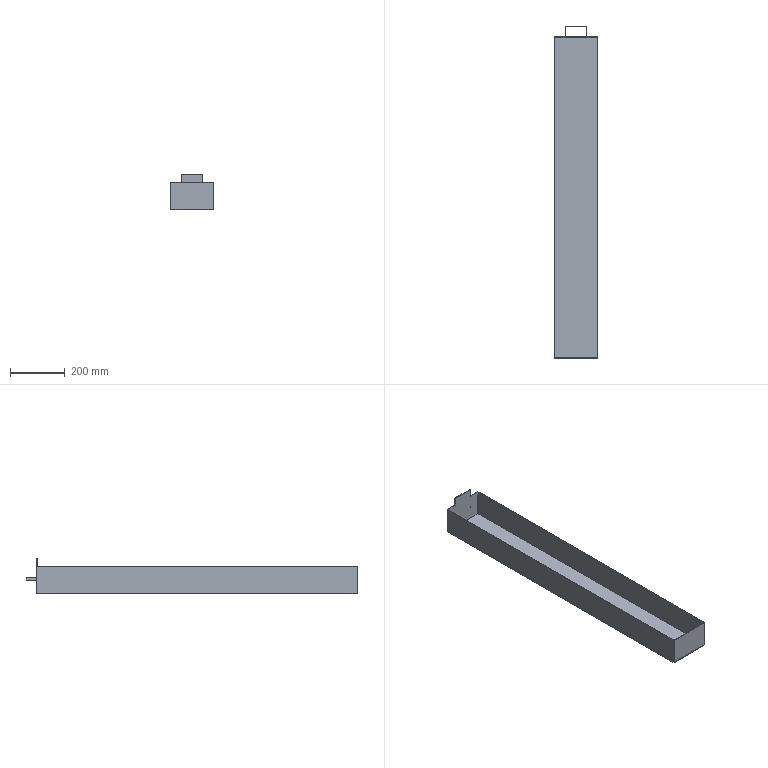Part | NX | features solid 2 | 1 solid | 22 faces | box 160 x 1212 x 130 mm | volume 903536 mm3 | plane 22
STEP:
#1=CARTESIAN_POINT('',(-370.,1107.,-565.));
#2=VERTEX_POINT('',#1);
#3=CARTESIAN_POINT('',(-370.,1107.,-465.));
#4=VERTEX_POINT('',#3);
#5=CARTESIAN_POINT('',(-370.,1107.,-565.));
#6=DIRECTION('',(0.,0.,1.));
#7=VECTOR('',#6,1000.);
#8=LINE('',#5,#7);
#9=EDGE_CURVE('',#2,#4,#8,.T.);
#10=ORIENTED_EDGE('',*,*,#9,.T.);
#11=CARTESIAN_POINT('',(-370.,-65.,-465.));
#12=VERTEX_POINT('',#11);
#13=CARTESIAN_POINT('',(-370.,807.,-465.));
#14=DIRECTION('',(0.,1.,0.));
#15=VECTOR('',#14,1000.);
#16=LINE('',#13,#15);
#17=EDGE_CURVE('',#12,#4,#16,.T.);
#18=ORIENTED_EDGE('',*,*,#17,.F.);
#19=CARTESIAN_POINT('',(-370.,-65.,-565.));
#20=VERTEX_POINT('',#19);
#21=CARTESIAN_POINT('',(-370.,-65.,-565.));
#22=DIRECTION('',(0.,0.,-1.));
#23=VECTOR('',#22,1000.);
#24=LINE('',#21,#23);
#25=EDGE_CURVE('',#20,#12,#24,.F.);
#26=ORIENTED_EDGE('',*,*,#25,.F.);
#27=CARTESIAN_POINT('',(-370.,807.,-565.));
#28=DIRECTION('',(0.,1.,0.));
#29=VECTOR('',#28,1000.);
#30=LINE('',#27,#29);
#31=EDGE_CURVE('',#20,#2,#30,.T.);
#32=ORIENTED_EDGE('',*,*,#31,.T.);
#33=EDGE_LOOP('',(#10,#18,#26,#32));
#34=FACE_BOUND('',#33,.T.);
#35=CARTESIAN_POINT('',(-370.,807.,-565.));
#36=DIRECTION('',(-1.,0.,0.));
#37=DIRECTION('',(0.,1.,0.));
#38=AXIS2_PLACEMENT_3D('',#35,#36,#37);
#39=PLANE('',#38);
#40=ADVANCED_FACE('',(#34),#39,.F.);
#41=CARTESIAN_POINT('',(-490.,1107.,-505.));
#42=VERTEX_POINT('',#41);
#43=CARTESIAN_POINT('',(-490.,1107.,-515.));
#44=VERTEX_POINT('',#43);
#45=CARTESIAN_POINT('',(-490.,1107.,-565.));
#46=DIRECTION('',(0.,0.,-1.));
#47=VECTOR('',#46,1000.);
#48=LINE('',#45,#47);
#49=EDGE_CURVE('',#42,#44,#48,.T.);
#50=ORIENTED_EDGE('',*,*,#49,.T.);
#51=CARTESIAN_POINT('',(-488.,1107.,-515.));
#52=VERTEX_POINT('',#51);
#53=CARTESIAN_POINT('',(-410.,1107.,-515.));
#54=DIRECTION('',(1.,0.,0.));
#55=VECTOR('',#54,1000.);
#56=LINE('',#53,#55);
#57=EDGE_CURVE('',#52,#44,#56,.F.);
#58=ORIENTED_EDGE('',*,*,#57,.F.);
#59=CARTESIAN_POINT('',(-488.,1107.,-505.));
#60=VERTEX_POINT('',#59);
#61=CARTESIAN_POINT('',(-488.,1107.,-565.));
#62=DIRECTION('',(0.,0.,-1.));
#63=VECTOR('',#62,1000.);
#64=LINE('',#61,#63);
#65=EDGE_CURVE('',#60,#52,#64,.T.);
#66=ORIENTED_EDGE('',*,*,#65,.F.);
#67=CARTESIAN_POINT('',(-410.,1107.,-505.));
#68=DIRECTION('',(1.,0.,0.));
#69=VECTOR('',#68,1000.);
#70=LINE('',#67,#69);
#71=EDGE_CURVE('',#60,#42,#70,.F.);
#72=ORIENTED_EDGE('',*,*,#71,.T.);
#73=EDGE_LOOP('',(#50,#58,#66,#72));
#74=FACE_BOUND('',#73,.T.);
#75=CARTESIAN_POINT('',(-412.,1107.,-505.));
#76=VERTEX_POINT('',#75);
#77=CARTESIAN_POINT('',(-412.,1107.,-515.));
#78=VERTEX_POINT('',#77);
#79=CARTESIAN_POINT('',(-412.,1107.,-565.));
#80=DIRECTION('',(0.,0.,1.));
#81=VECTOR('',#80,1000.);
#82=LINE('',#79,#81);
#83=EDGE_CURVE('',#76,#78,#82,.F.);
#84=ORIENTED_EDGE('',*,*,#83,.T.);
#85=CARTESIAN_POINT('',(-410.,1107.,-515.));
#86=VERTEX_POINT('',#85);
#87=CARTESIAN_POINT('',(-410.,1107.,-515.));
#88=DIRECTION('',(1.,0.,0.));
#89=VECTOR('',#88,1000.);
#90=LINE('',#87,#89);
#91=EDGE_CURVE('',#86,#78,#90,.F.);
#92=ORIENTED_EDGE('',*,*,#91,.F.);
#93=CARTESIAN_POINT('',(-410.,1107.,-505.));
#94=VERTEX_POINT('',#93);
#95=CARTESIAN_POINT('',(-410.,1107.,-565.));
#96=DIRECTION('',(0.,0.,-1.));
#97=VECTOR('',#96,1000.);
#98=LINE('',#95,#97);
#99=EDGE_CURVE('',#94,#86,#98,.T.);
#100=ORIENTED_EDGE('',*,*,#99,.F.);
#101=CARTESIAN_POINT('',(-410.,1107.,-505.));
#102=DIRECTION('',(1.,0.,0.));
#103=VECTOR('',#102,1000.);
#104=LINE('',#101,#103);
#105=EDGE_CURVE('',#94,#76,#104,.F.);
#106=ORIENTED_EDGE('',*,*,#105,.T.);
#107=EDGE_LOOP('',(#84,#92,#100,#106));
#108=FACE_BOUND('',#107,.T.);
#109=CARTESIAN_POINT('',(-410.,1107.,-465.));
#110=VERTEX_POINT('',#109);
#111=CARTESIAN_POINT('',(-375.,1107.,-465.));
#112=DIRECTION('',(-1.,0.,0.));
#113=VECTOR('',#112,1000.);
#114=LINE('',#111,#113);
#115=EDGE_CURVE('',#4,#110,#114,.T.);
#116=ORIENTED_EDGE('',*,*,#115,.F.);
#117=ORIENTED_EDGE('',*,*,#9,.F.);
#118=CARTESIAN_POINT('',(-530.,1107.,-565.));
#119=VERTEX_POINT('',#118);
#120=CARTESIAN_POINT('',(-375.,1107.,-565.));
#121=DIRECTION('',(-1.,0.,0.));
#122=VECTOR('',#121,1000.);
#123=LINE('',#120,#122);
#124=EDGE_CURVE('',#2,#119,#123,.T.);
#125=ORIENTED_EDGE('',*,*,#124,.T.);
#126=CARTESIAN_POINT('',(-530.,1107.,-465.));
#127=VERTEX_POINT('',#126);
#128=CARTESIAN_POINT('',(-530.,1107.,-565.));
#129=DIRECTION('',(0.,0.,-1.));
#130=VECTOR('',#129,1000.);
#131=LINE('',#128,#130);
#132=EDGE_CURVE('',#119,#127,#131,.F.);
#133=ORIENTED_EDGE('',*,*,#132,.T.);
#134=CARTESIAN_POINT('',(-490.,1107.,-465.));
#135=VERTEX_POINT('',#134);
#136=CARTESIAN_POINT('',(-375.,1107.,-465.));
#137=DIRECTION('',(-1.,0.,0.));
#138=VECTOR('',#137,1000.);
#139=LINE('',#136,#138);
#140=EDGE_CURVE('',#135,#127,#139,.T.);
#141=ORIENTED_EDGE('',*,*,#140,.F.);
#142=CARTESIAN_POINT('',(-490.,1107.,-435.));
#143=VERTEX_POINT('',#142);
#144=CARTESIAN_POINT('',(-490.,1107.,-565.));
#145=DIRECTION('',(0.,0.,-1.));
#146=VECTOR('',#145,1000.);
#147=LINE('',#144,#146);
#148=EDGE_CURVE('',#135,#143,#147,.F.);
#149=ORIENTED_EDGE('',*,*,#148,.T.);
#150=CARTESIAN_POINT('',(-410.,1107.,-435.));
#151=VERTEX_POINT('',#150);
#152=CARTESIAN_POINT('',(-370.,1107.,-435.));
#153=DIRECTION('',(-1.,0.,0.));
#154=VECTOR('',#153,1000.);
#155=LINE('',#152,#154);
#156=EDGE_CURVE('',#151,#143,#155,.T.);
#157=ORIENTED_EDGE('',*,*,#156,.F.);
#158=CARTESIAN_POINT('',(-410.,1107.,-565.));
#159=DIRECTION('',(0.,0.,1.));
#160=VECTOR('',#159,1000.);
#161=LINE('',#158,#160);
#162=EDGE_CURVE('',#110,#151,#161,.T.);
#163=ORIENTED_EDGE('',*,*,#162,.F.);
#164=EDGE_LOOP('',(#116,#117,#125,#133,#141,#149,#157,#163));
#165=FACE_BOUND('',#164,.T.);
#166=CARTESIAN_POINT('',(-375.,1107.,-565.));
#167=DIRECTION('',(0.,-1.,0.));
#168=DIRECTION('',(-1.,0.,0.));
#169=AXIS2_PLACEMENT_3D('',#166,#167,#168);
#170=PLANE('',#169);
#171=ADVANCED_FACE('',(#74,#108,#165),#170,.F.);
#172=CARTESIAN_POINT('',(-530.,-65.,-465.));
#173=VERTEX_POINT('',#172);
#174=CARTESIAN_POINT('',(-530.,807.,-465.));
#175=DIRECTION('',(0.,-1.,0.));
#176=VECTOR('',#175,1000.);
#177=LINE('',#174,#176);
#178=EDGE_CURVE('',#173,#127,#177,.F.);
#179=ORIENTED_EDGE('',*,*,#178,.T.);
#180=ORIENTED_EDGE('',*,*,#132,.F.);
#181=CARTESIAN_POINT('',(-530.,-65.,-565.));
#182=VERTEX_POINT('',#181);
#183=CARTESIAN_POINT('',(-530.,807.,-565.));
#184=DIRECTION('',(0.,-1.,0.));
#185=VECTOR('',#184,1000.);
#186=LINE('',#183,#185);
#187=EDGE_CURVE('',#182,#119,#186,.F.);
#188=ORIENTED_EDGE('',*,*,#187,.F.);
#189=CARTESIAN_POINT('',(-530.,-65.,-565.));
#190=DIRECTION('',(0.,0.,1.));
#191=VECTOR('',#190,1000.);
#192=LINE('',#189,#191);
#193=EDGE_CURVE('',#182,#173,#192,.T.);
#194=ORIENTED_EDGE('',*,*,#193,.T.);
#195=EDGE_LOOP('',(#179,#180,#188,#194));
#196=FACE_BOUND('',#195,.T.);
#197=CARTESIAN_POINT('',(-530.,807.,-565.));
#198=DIRECTION('',(-1.,0.,0.));
#199=DIRECTION('',(0.,1.,0.));
#200=AXIS2_PLACEMENT_3D('',#197,#198,#199);
#201=PLANE('',#200);
#202=ADVANCED_FACE('',(#196),#201,.T.);
#203=CARTESIAN_POINT('',(-372.,1105.,-563.));
#204=VERTEX_POINT('',#203);
#205=CARTESIAN_POINT('',(-372.,1105.,-465.));
#206=VERTEX_POINT('',#205);
#207=CARTESIAN_POINT('',(-372.,1105.,-565.));
#208=DIRECTION('',(0.,0.,1.));
#209=VECTOR('',#208,1000.);
#210=LINE('',#207,#209);
#211=EDGE_CURVE('',#204,#206,#210,.T.);
#212=ORIENTED_EDGE('',*,*,#211,.T.);
#213=CARTESIAN_POINT('',(-410.,1105.,-465.));
#214=VERTEX_POINT('',#213);
#215=CARTESIAN_POINT('',(-375.,1105.,-465.));
#216=DIRECTION('',(-1.,0.,0.));
#217=VECTOR('',#216,1000.);
#218=LINE('',#215,#217);
#219=EDGE_CURVE('',#206,#214,#218,.T.);
#220=ORIENTED_EDGE('',*,*,#219,.T.);
#221=CARTESIAN_POINT('',(-410.,1105.,-435.));
#222=VERTEX_POINT('',#221);
#223=CARTESIAN_POINT('',(-410.,1105.,-565.));
#224=DIRECTION('',(0.,0.,1.));
#225=VECTOR('',#224,1000.);
#226=LINE('',#223,#225);
#227=EDGE_CURVE('',#214,#222,#226,.T.);
#228=ORIENTED_EDGE('',*,*,#227,.T.);
#229=CARTESIAN_POINT('',(-490.,1105.,-435.));
#230=VERTEX_POINT('',#229);
#231=CARTESIAN_POINT('',(-370.,1105.,-435.));
#232=DIRECTION('',(-1.,0.,0.));
#233=VECTOR('',#232,1000.);
#234=LINE('',#231,#233);
#235=EDGE_CURVE('',#222,#230,#234,.T.);
#236=ORIENTED_EDGE('',*,*,#235,.T.);
#237=CARTESIAN_POINT('',(-490.,1105.,-465.));
#238=VERTEX_POINT('',#237);
#239=CARTESIAN_POINT('',(-490.,1105.,-565.));
#240=DIRECTION('',(0.,0.,-1.));
#241=VECTOR('',#240,1000.);
#242=LINE('',#239,#241);
#243=EDGE_CURVE('',#238,#230,#242,.F.);
#244=ORIENTED_EDGE('',*,*,#243,.F.);
#245=CARTESIAN_POINT('',(-528.,1105.,-465.));
#246=VERTEX_POINT('',#245);
#247=CARTESIAN_POINT('',(-375.,1105.,-465.));
#248=DIRECTION('',(-1.,0.,0.));
#249=VECTOR('',#248,1000.);
#250=LINE('',#247,#249);
#251=EDGE_CURVE('',#238,#246,#250,.T.);
#252=ORIENTED_EDGE('',*,*,#251,.T.);
#253=CARTESIAN_POINT('',(-528.,1105.,-563.));
#254=VERTEX_POINT('',#253);
#255=CARTESIAN_POINT('',(-528.,1105.,-565.));
#256=DIRECTION('',(0.,0.,-1.));
#257=VECTOR('',#256,1000.);
#258=LINE('',#255,#257);
#259=EDGE_CURVE('',#254,#246,#258,.F.);
#260=ORIENTED_EDGE('',*,*,#259,.F.);
#261=CARTESIAN_POINT('',(-375.,1105.,-563.));
#262=DIRECTION('',(-1.,0.,0.));
#263=VECTOR('',#262,1000.);
#264=LINE('',#261,#263);
#265=EDGE_CURVE('',#204,#254,#264,.T.);
#266=ORIENTED_EDGE('',*,*,#265,.F.);
#267=EDGE_LOOP('',(#212,#220,#228,#236,#244,#252,#260,#266));
#268=FACE_BOUND('',#267,.T.);
#269=CARTESIAN_POINT('',(-375.,1105.,-565.));
#270=DIRECTION('',(0.,-1.,0.));
#271=DIRECTION('',(-1.,0.,0.));
#272=AXIS2_PLACEMENT_3D('',#269,#270,#271);
#273=PLANE('',#272);
#274=ADVANCED_FACE('',(#268),#273,.T.);
#275=CARTESIAN_POINT('',(-490.,807.,-465.));
#276=DIRECTION('',(0.,1.,0.));
#277=VECTOR('',#276,1000.);
#278=LINE('',#275,#277);
#279=EDGE_CURVE('',#135,#238,#278,.F.);
#280=ORIENTED_EDGE('',*,*,#279,.F.);
#281=ORIENTED_EDGE('',*,*,#140,.T.);
#282=ORIENTED_EDGE('',*,*,#178,.F.);
#283=CARTESIAN_POINT('',(-375.,-65.,-465.));
#284=DIRECTION('',(1.,0.,0.));
#285=VECTOR('',#284,1000.);
#286=LINE('',#283,#285);
#287=EDGE_CURVE('',#12,#173,#286,.F.);
#288=ORIENTED_EDGE('',*,*,#287,.F.);
#289=ORIENTED_EDGE('',*,*,#17,.T.);
#290=ORIENTED_EDGE('',*,*,#115,.T.);
#291=CARTESIAN_POINT('',(-410.,807.,-465.));
#292=DIRECTION('',(0.,1.,0.));
#293=VECTOR('',#292,1000.);
#294=LINE('',#291,#293);
#295=EDGE_CURVE('',#214,#110,#294,.T.);
#296=ORIENTED_EDGE('',*,*,#295,.F.);
#297=ORIENTED_EDGE('',*,*,#219,.F.);
#298=CARTESIAN_POINT('',(-372.,-63.,-465.));
#299=VERTEX_POINT('',#298);
#300=CARTESIAN_POINT('',(-372.,807.,-465.));
#301=DIRECTION('',(0.,1.,0.));
#302=VECTOR('',#301,1000.);
#303=LINE('',#300,#302);
#304=EDGE_CURVE('',#299,#206,#303,.T.);
#305=ORIENTED_EDGE('',*,*,#304,.F.);
#306=CARTESIAN_POINT('',(-528.,-63.,-465.));
#307=VERTEX_POINT('',#306);
#308=CARTESIAN_POINT('',(-375.,-63.,-465.));
#309=DIRECTION('',(1.,0.,0.));
#310=VECTOR('',#309,1000.);
#311=LINE('',#308,#310);
#312=EDGE_CURVE('',#299,#307,#311,.F.);
#313=ORIENTED_EDGE('',*,*,#312,.T.);
#314=CARTESIAN_POINT('',(-528.,807.,-465.));
#315=DIRECTION('',(0.,-1.,0.));
#316=VECTOR('',#315,1000.);
#317=LINE('',#314,#316);
#318=EDGE_CURVE('',#307,#246,#317,.F.);
#319=ORIENTED_EDGE('',*,*,#318,.T.);
#320=ORIENTED_EDGE('',*,*,#251,.F.);
#321=EDGE_LOOP('',(#280,#281,#282,#288,#289,#290,#296,#297,#305,#313,#319,#320));
#322=FACE_BOUND('',#321,.T.);
#323=CARTESIAN_POINT('',(-375.,807.,-465.));
#324=DIRECTION('',(0.,0.,1.));
#325=DIRECTION('',(1.,0.,0.));
#326=AXIS2_PLACEMENT_3D('',#323,#324,#325);
#327=PLANE('',#326);
#328=ADVANCED_FACE('',(#322),#327,.T.);
#329=ORIENTED_EDGE('',*,*,#31,.F.);
#330=CARTESIAN_POINT('',(-375.,-65.,-565.));
#331=DIRECTION('',(1.,0.,0.));
#332=VECTOR('',#331,1000.);
#333=LINE('',#330,#332);
#334=EDGE_CURVE('',#20,#182,#333,.F.);
#335=ORIENTED_EDGE('',*,*,#334,.T.);
#336=ORIENTED_EDGE('',*,*,#187,.T.);
#337=ORIENTED_EDGE('',*,*,#124,.F.);
#338=EDGE_LOOP('',(#329,#335,#336,#337));
#339=FACE_BOUND('',#338,.T.);
#340=CARTESIAN_POINT('',(-375.,807.,-565.));
#341=DIRECTION('',(0.,0.,1.));
#342=DIRECTION('',(1.,0.,0.));
#343=AXIS2_PLACEMENT_3D('',#340,#341,#342);
#344=PLANE('',#343);
#345=ADVANCED_FACE('',(#339),#344,.F.);
#346=CARTESIAN_POINT('',(-372.,-63.,-563.));
#347=VERTEX_POINT('',#346);
#348=CARTESIAN_POINT('',(-372.,807.,-563.));
#349=DIRECTION('',(0.,1.,0.));
#350=VECTOR('',#349,1000.);
#351=LINE('',#348,#350);
#352=EDGE_CURVE('',#347,#204,#351,.T.);
#353=ORIENTED_EDGE('',*,*,#352,.F.);
#354=CARTESIAN_POINT('',(-372.,-63.,-565.));
#355=DIRECTION('',(0.,0.,-1.));
#356=VECTOR('',#355,1000.);
#357=LINE('',#354,#356);
#358=EDGE_CURVE('',#347,#299,#357,.F.);
#359=ORIENTED_EDGE('',*,*,#358,.T.);
#360=ORIENTED_EDGE('',*,*,#304,.T.);
#361=ORIENTED_EDGE('',*,*,#211,.F.);
#362=EDGE_LOOP('',(#353,#359,#360,#361));
#363=FACE_BOUND('',#362,.T.);
#364=CARTESIAN_POINT('',(-372.,807.,-565.));
#365=DIRECTION('',(-1.,0.,0.));
#366=DIRECTION('',(0.,1.,0.));
#367=AXIS2_PLACEMENT_3D('',#364,#365,#366);
#368=PLANE('',#367);
#369=ADVANCED_FACE('',(#363),#368,.T.);
#370=ORIENTED_EDGE('',*,*,#318,.F.);
#371=CARTESIAN_POINT('',(-528.,-63.,-563.));
#372=VERTEX_POINT('',#371);
#373=CARTESIAN_POINT('',(-528.,-63.,-565.));
#374=DIRECTION('',(0.,0.,1.));
#375=VECTOR('',#374,1000.);
#376=LINE('',#373,#375);
#377=EDGE_CURVE('',#372,#307,#376,.T.);
#378=ORIENTED_EDGE('',*,*,#377,.F.);
#379=CARTESIAN_POINT('',(-528.,807.,-563.));
#380=DIRECTION('',(0.,-1.,0.));
#381=VECTOR('',#380,1000.);
#382=LINE('',#379,#381);
#383=EDGE_CURVE('',#372,#254,#382,.F.);
#384=ORIENTED_EDGE('',*,*,#383,.T.);
#385=ORIENTED_EDGE('',*,*,#259,.T.);
#386=EDGE_LOOP('',(#370,#378,#384,#385));
#387=FACE_BOUND('',#386,.T.);
#388=CARTESIAN_POINT('',(-528.,807.,-565.));
#389=DIRECTION('',(-1.,0.,0.));
#390=DIRECTION('',(0.,1.,0.));
#391=AXIS2_PLACEMENT_3D('',#388,#389,#390);
#392=PLANE('',#391);
#393=ADVANCED_FACE('',(#387),#392,.F.);
#394=ORIENTED_EDGE('',*,*,#383,.F.);
#395=CARTESIAN_POINT('',(-375.,-63.,-563.));
#396=DIRECTION('',(1.,0.,0.));
#397=VECTOR('',#396,1000.);
#398=LINE('',#395,#397);
#399=EDGE_CURVE('',#347,#372,#398,.F.);
#400=ORIENTED_EDGE('',*,*,#399,.F.);
#401=ORIENTED_EDGE('',*,*,#352,.T.);
#402=ORIENTED_EDGE('',*,*,#265,.T.);
#403=EDGE_LOOP('',(#394,#400,#401,#402));
#404=FACE_BOUND('',#403,.T.);
#405=CARTESIAN_POINT('',(-375.,807.,-563.));
#406=DIRECTION('',(0.,0.,1.));
#407=DIRECTION('',(1.,0.,0.));
#408=AXIS2_PLACEMENT_3D('',#405,#406,#407);
#409=PLANE('',#408);
#410=ADVANCED_FACE('',(#404),#409,.T.);
#411=ORIENTED_EDGE('',*,*,#105,.F.);
#412=CARTESIAN_POINT('',(-410.,1147.,-505.));
#413=VERTEX_POINT('',#412);
#414=CARTESIAN_POINT('',(-410.,1107.,-505.));
#415=DIRECTION('',(0.,-1.,0.));
#416=VECTOR('',#415,1000.);
#417=LINE('',#414,#416);
#418=EDGE_CURVE('',#94,#413,#417,.F.);
#419=ORIENTED_EDGE('',*,*,#418,.T.);
#420=CARTESIAN_POINT('',(-490.,1147.,-505.));
#421=VERTEX_POINT('',#420);
#422=CARTESIAN_POINT('',(-410.,1147.,-505.));
#423=DIRECTION('',(1.,0.,0.));
#424=VECTOR('',#423,1000.);
#425=LINE('',#422,#424);
#426=EDGE_CURVE('',#413,#421,#425,.F.);
#427=ORIENTED_EDGE('',*,*,#426,.T.);
#428=CARTESIAN_POINT('',(-490.,1107.,-505.));
#429=DIRECTION('',(0.,-1.,0.));
#430=VECTOR('',#429,1000.);
#431=LINE('',#428,#430);
#432=EDGE_CURVE('',#42,#421,#431,.F.);
#433=ORIENTED_EDGE('',*,*,#432,.F.);
#434=ORIENTED_EDGE('',*,*,#71,.F.);
#435=CARTESIAN_POINT('',(-488.,1145.,-505.));
#436=VERTEX_POINT('',#435);
#437=CARTESIAN_POINT('',(-488.,1107.,-505.));
#438=DIRECTION('',(0.,1.,0.));
#439=VECTOR('',#438,1000.);
#440=LINE('',#437,#439);
#441=EDGE_CURVE('',#60,#436,#440,.T.);
#442=ORIENTED_EDGE('',*,*,#441,.T.);
#443=CARTESIAN_POINT('',(-412.,1145.,-505.));
#444=VERTEX_POINT('',#443);
#445=CARTESIAN_POINT('',(-410.,1145.,-505.));
#446=DIRECTION('',(1.,0.,0.));
#447=VECTOR('',#446,1000.);
#448=LINE('',#445,#447);
#449=EDGE_CURVE('',#444,#436,#448,.F.);
#450=ORIENTED_EDGE('',*,*,#449,.F.);
#451=CARTESIAN_POINT('',(-412.,1107.,-505.));
#452=DIRECTION('',(0.,-1.,0.));
#453=VECTOR('',#452,1000.);
#454=LINE('',#451,#453);
#455=EDGE_CURVE('',#76,#444,#454,.F.);
#456=ORIENTED_EDGE('',*,*,#455,.F.);
#457=EDGE_LOOP('',(#411,#419,#427,#433,#434,#442,#450,#456));
#458=FACE_BOUND('',#457,.T.);
#459=CARTESIAN_POINT('',(-410.,1107.,-505.));
#460=DIRECTION('',(0.,0.,1.));
#461=DIRECTION('',(1.,0.,0.));
#462=AXIS2_PLACEMENT_3D('',#459,#460,#461);
#463=PLANE('',#462);
#464=ADVANCED_FACE('',(#458),#463,.T.);
#465=ORIENTED_EDGE('',*,*,#99,.T.);
#466=CARTESIAN_POINT('',(-410.,1147.,-515.));
#467=VERTEX_POINT('',#466);
#468=CARTESIAN_POINT('',(-410.,1107.,-515.));
#469=DIRECTION('',(0.,-1.,0.));
#470=VECTOR('',#469,1000.);
#471=LINE('',#468,#470);
#472=EDGE_CURVE('',#86,#467,#471,.F.);
#473=ORIENTED_EDGE('',*,*,#472,.T.);
#474=CARTESIAN_POINT('',(-410.,1147.,-565.));
#475=DIRECTION('',(0.,0.,-1.));
#476=VECTOR('',#475,1000.);
#477=LINE('',#474,#476);
#478=EDGE_CURVE('',#413,#467,#477,.T.);
#479=ORIENTED_EDGE('',*,*,#478,.F.);
#480=ORIENTED_EDGE('',*,*,#418,.F.);
#481=EDGE_LOOP('',(#465,#473,#479,#480));
#482=FACE_BOUND('',#481,.T.);
#483=CARTESIAN_POINT('',(-410.,1107.,-565.));
#484=DIRECTION('',(-1.,0.,0.));
#485=DIRECTION('',(0.,1.,0.));
#486=AXIS2_PLACEMENT_3D('',#483,#484,#485);
#487=PLANE('',#486);
#488=ADVANCED_FACE('',(#482),#487,.F.);
#489=ORIENTED_EDGE('',*,*,#478,.T.);
#490=CARTESIAN_POINT('',(-490.,1147.,-515.));
#491=VERTEX_POINT('',#490);
#492=CARTESIAN_POINT('',(-410.,1147.,-515.));
#493=DIRECTION('',(1.,0.,0.));
#494=VECTOR('',#493,1000.);
#495=LINE('',#492,#494);
#496=EDGE_CURVE('',#467,#491,#495,.F.);
#497=ORIENTED_EDGE('',*,*,#496,.T.);
#498=CARTESIAN_POINT('',(-490.,1147.,-565.));
#499=DIRECTION('',(0.,0.,-1.));
#500=VECTOR('',#499,1000.);
#501=LINE('',#498,#500);
#502=EDGE_CURVE('',#421,#491,#501,.T.);
#503=ORIENTED_EDGE('',*,*,#502,.F.);
#504=ORIENTED_EDGE('',*,*,#426,.F.);
#505=EDGE_LOOP('',(#489,#497,#503,#504));
#506=FACE_BOUND('',#505,.T.);
#507=CARTESIAN_POINT('',(-410.,1147.,-565.));
#508=DIRECTION('',(0.,-1.,0.));
#509=DIRECTION('',(-1.,0.,0.));
#510=AXIS2_PLACEMENT_3D('',#507,#508,#509);
#511=PLANE('',#510);
#512=ADVANCED_FACE('',(#506),#511,.F.);
#513=ORIENTED_EDGE('',*,*,#432,.T.);
#514=ORIENTED_EDGE('',*,*,#502,.T.);
#515=CARTESIAN_POINT('',(-490.,1107.,-515.));
#516=DIRECTION('',(0.,-1.,0.));
#517=VECTOR('',#516,1000.);
#518=LINE('',#515,#517);
#519=EDGE_CURVE('',#44,#491,#518,.F.);
#520=ORIENTED_EDGE('',*,*,#519,.F.);
#521=ORIENTED_EDGE('',*,*,#49,.F.);
#522=EDGE_LOOP('',(#513,#514,#520,#521));
#523=FACE_BOUND('',#522,.T.);
#524=CARTESIAN_POINT('',(-490.,1107.,-565.));
#525=DIRECTION('',(-1.,0.,0.));
#526=DIRECTION('',(0.,1.,0.));
#527=AXIS2_PLACEMENT_3D('',#524,#525,#526);
#528=PLANE('',#527);
#529=ADVANCED_FACE('',(#523),#528,.T.);
#530=ORIENTED_EDGE('',*,*,#57,.T.);
#531=ORIENTED_EDGE('',*,*,#519,.T.);
#532=ORIENTED_EDGE('',*,*,#496,.F.);
#533=ORIENTED_EDGE('',*,*,#472,.F.);
#534=ORIENTED_EDGE('',*,*,#91,.T.);
#535=CARTESIAN_POINT('',(-412.,1145.,-515.));
#536=VERTEX_POINT('',#535);
#537=CARTESIAN_POINT('',(-412.,1107.,-515.));
#538=DIRECTION('',(0.,-1.,0.));
#539=VECTOR('',#538,1000.);
#540=LINE('',#537,#539);
#541=EDGE_CURVE('',#78,#536,#540,.F.);
#542=ORIENTED_EDGE('',*,*,#541,.T.);
#543=CARTESIAN_POINT('',(-488.,1145.,-515.));
#544=VERTEX_POINT('',#543);
#545=CARTESIAN_POINT('',(-410.,1145.,-515.));
#546=DIRECTION('',(1.,0.,0.));
#547=VECTOR('',#546,1000.);
#548=LINE('',#545,#547);
#549=EDGE_CURVE('',#536,#544,#548,.F.);
#550=ORIENTED_EDGE('',*,*,#549,.T.);
#551=CARTESIAN_POINT('',(-488.,1107.,-515.));
#552=DIRECTION('',(0.,1.,0.));
#553=VECTOR('',#552,1000.);
#554=LINE('',#551,#553);
#555=EDGE_CURVE('',#52,#544,#554,.T.);
#556=ORIENTED_EDGE('',*,*,#555,.F.);
#557=EDGE_LOOP('',(#530,#531,#532,#533,#534,#542,#550,#556));
#558=FACE_BOUND('',#557,.T.);
#559=CARTESIAN_POINT('',(-410.,1107.,-515.));
#560=DIRECTION('',(0.,0.,1.));
#561=DIRECTION('',(1.,0.,0.));
#562=AXIS2_PLACEMENT_3D('',#559,#560,#561);
#563=PLANE('',#562);
#564=ADVANCED_FACE('',(#558),#563,.F.);
#565=ORIENTED_EDGE('',*,*,#83,.F.);
#566=ORIENTED_EDGE('',*,*,#455,.T.);
#567=CARTESIAN_POINT('',(-412.,1145.,-565.));
#568=DIRECTION('',(0.,0.,-1.));
#569=VECTOR('',#568,1000.);
#570=LINE('',#567,#569);
#571=EDGE_CURVE('',#444,#536,#570,.T.);
#572=ORIENTED_EDGE('',*,*,#571,.T.);
#573=ORIENTED_EDGE('',*,*,#541,.F.);
#574=EDGE_LOOP('',(#565,#566,#572,#573));
#575=FACE_BOUND('',#574,.T.);
#576=CARTESIAN_POINT('',(-412.,1107.,-565.));
#577=DIRECTION('',(-1.,0.,0.));
#578=DIRECTION('',(0.,1.,0.));
#579=AXIS2_PLACEMENT_3D('',#576,#577,#578);
#580=PLANE('',#579);
#581=ADVANCED_FACE('',(#575),#580,.T.);
#582=ORIENTED_EDGE('',*,*,#571,.F.);
#583=ORIENTED_EDGE('',*,*,#449,.T.);
#584=CARTESIAN_POINT('',(-488.,1145.,-565.));
#585=DIRECTION('',(0.,0.,1.));
#586=VECTOR('',#585,1000.);
#587=LINE('',#584,#586);
#588=EDGE_CURVE('',#436,#544,#587,.F.);
#589=ORIENTED_EDGE('',*,*,#588,.T.);
#590=ORIENTED_EDGE('',*,*,#549,.F.);
#591=EDGE_LOOP('',(#582,#583,#589,#590));
#592=FACE_BOUND('',#591,.T.);
#593=CARTESIAN_POINT('',(-410.,1145.,-565.));
#594=DIRECTION('',(0.,-1.,0.));
#595=DIRECTION('',(-1.,0.,0.));
#596=AXIS2_PLACEMENT_3D('',#593,#594,#595);
#597=PLANE('',#596);
#598=ADVANCED_FACE('',(#592),#597,.T.);
#599=ORIENTED_EDGE('',*,*,#441,.F.);
#600=ORIENTED_EDGE('',*,*,#65,.T.);
#601=ORIENTED_EDGE('',*,*,#555,.T.);
#602=ORIENTED_EDGE('',*,*,#588,.F.);
#603=EDGE_LOOP('',(#599,#600,#601,#602));
#604=FACE_BOUND('',#603,.T.);
#605=CARTESIAN_POINT('',(-488.,1107.,-565.));
#606=DIRECTION('',(-1.,0.,0.));
#607=DIRECTION('',(0.,1.,0.));
#608=AXIS2_PLACEMENT_3D('',#605,#606,#607);
#609=PLANE('',#608);
#610=ADVANCED_FACE('',(#604),#609,.F.);
#611=ORIENTED_EDGE('',*,*,#193,.F.);
#612=ORIENTED_EDGE('',*,*,#334,.F.);
#613=ORIENTED_EDGE('',*,*,#25,.T.);
#614=ORIENTED_EDGE('',*,*,#287,.T.);
#615=EDGE_LOOP('',(#611,#612,#613,#614));
#616=FACE_BOUND('',#615,.T.);
#617=CARTESIAN_POINT('',(-375.,-65.,-565.));
#618=DIRECTION('',(0.,-1.,0.));
#619=DIRECTION('',(-1.,0.,0.));
#620=AXIS2_PLACEMENT_3D('',#617,#618,#619);
#621=PLANE('',#620);
#622=ADVANCED_FACE('',(#616),#621,.T.);
#623=ORIENTED_EDGE('',*,*,#377,.T.);
#624=ORIENTED_EDGE('',*,*,#312,.F.);
#625=ORIENTED_EDGE('',*,*,#358,.F.);
#626=ORIENTED_EDGE('',*,*,#399,.T.);
#627=EDGE_LOOP('',(#623,#624,#625,#626));
#628=FACE_BOUND('',#627,.T.);
#629=CARTESIAN_POINT('',(-375.,-63.,-565.));
#630=DIRECTION('',(0.,-1.,0.));
#631=DIRECTION('',(-1.,0.,0.));
#632=AXIS2_PLACEMENT_3D('',#629,#630,#631);
#633=PLANE('',#632);
#634=ADVANCED_FACE('',(#628),#633,.F.);
#635=ORIENTED_EDGE('',*,*,#235,.F.);
#636=CARTESIAN_POINT('',(-410.,807.,-435.));
#637=DIRECTION('',(0.,-1.,0.));
#638=VECTOR('',#637,1000.);
#639=LINE('',#636,#638);
#640=EDGE_CURVE('',#151,#222,#639,.T.);
#641=ORIENTED_EDGE('',*,*,#640,.F.);
#642=ORIENTED_EDGE('',*,*,#156,.T.);
#643=CARTESIAN_POINT('',(-490.,1107.,-435.));
#644=DIRECTION('',(0.,1.,0.));
#645=VECTOR('',#644,1000.);
#646=LINE('',#643,#645);
#647=EDGE_CURVE('',#143,#230,#646,.F.);
#648=ORIENTED_EDGE('',*,*,#647,.T.);
#649=EDGE_LOOP('',(#635,#641,#642,#648));
#650=FACE_BOUND('',#649,.T.);
#651=CARTESIAN_POINT('',(-370.,1107.,-435.));
#652=DIRECTION('',(0.,0.,-1.));
#653=DIRECTION('',(-1.,0.,0.));
#654=AXIS2_PLACEMENT_3D('',#651,#652,#653);
#655=PLANE('',#654);
#656=ADVANCED_FACE('',(#650),#655,.F.);
#657=ORIENTED_EDGE('',*,*,#148,.F.);
#658=ORIENTED_EDGE('',*,*,#279,.T.);
#659=ORIENTED_EDGE('',*,*,#243,.T.);
#660=ORIENTED_EDGE('',*,*,#647,.F.);
#661=EDGE_LOOP('',(#657,#658,#659,#660));
#662=FACE_BOUND('',#661,.T.);
#663=CARTESIAN_POINT('',(-490.,807.,-565.));
#664=DIRECTION('',(-1.,0.,0.));
#665=DIRECTION('',(0.,1.,0.));
#666=AXIS2_PLACEMENT_3D('',#663,#664,#665);
#667=PLANE('',#666);
#668=ADVANCED_FACE('',(#662),#667,.T.);
#669=ORIENTED_EDGE('',*,*,#227,.F.);
#670=ORIENTED_EDGE('',*,*,#295,.T.);
#671=ORIENTED_EDGE('',*,*,#162,.T.);
#672=ORIENTED_EDGE('',*,*,#640,.T.);
#673=EDGE_LOOP('',(#669,#670,#671,#672));
#674=FACE_BOUND('',#673,.T.);
#675=CARTESIAN_POINT('',(-410.,807.,-565.));
#676=DIRECTION('',(-1.,0.,0.));
#677=DIRECTION('',(0.,1.,0.));
#678=AXIS2_PLACEMENT_3D('',#675,#676,#677);
#679=PLANE('',#678);
#680=ADVANCED_FACE('',(#674),#679,.F.);
#681=CLOSED_SHELL('',(#40,#171,#202,#274,#328,#345,#369,#393,#410,#464,#488,#512,#529,#564,#581,#598,#610,#622,#634,#656,#668,#680));
#682=MANIFOLD_SOLID_BREP('',#681);
#683=(LENGTH_UNIT()NAMED_UNIT(*)SI_UNIT(.MILLI.,.METRE.));
#684=UNCERTAINTY_MEASURE_WITH_UNIT(LENGTH_MEASURE(0.00001),#683,'','');
#685=(NAMED_UNIT(*)PLANE_ANGLE_UNIT()SI_UNIT($,.RADIAN.));
#686=(NAMED_UNIT(*)SI_UNIT($,.STERADIAN.)SOLID_ANGLE_UNIT());
#687=(GEOMETRIC_REPRESENTATION_CONTEXT(3)GLOBAL_UNCERTAINTY_ASSIGNED_CONTEXT((#684))GLOBAL_UNIT_ASSIGNED_CONTEXT((#683,#685,#686))REPRESENTATION_CONTEXT('',''));
#688=ADVANCED_BREP_SHAPE_REPRESENTATION('',(#682),#687);